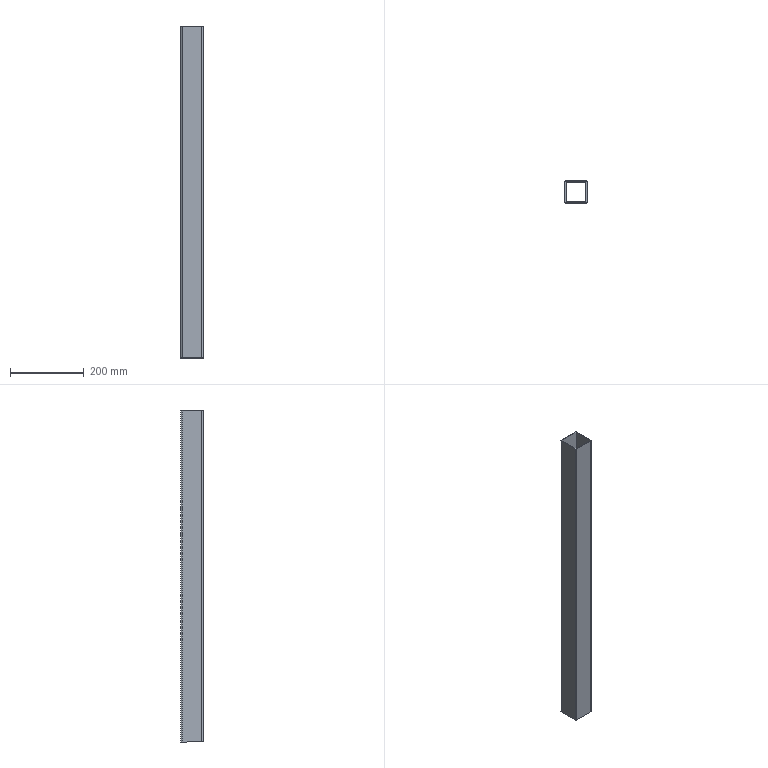Part | STEP file | X77-03102 | 1 solid | 14 faces | box 60 x 60 x 900 mm | volume 608647 mm3 | plane 10 | cylinder 4 | commonest cylinder face diameters 6 x4
STEP:
#1=CARTESIAN_POINT('',(0.,3.,900.));
#2=VERTEX_POINT('',#1);
#3=CARTESIAN_POINT('',(3.,0.,900.));
#4=VERTEX_POINT('',#3);
#5=CARTESIAN_POINT('',(3.,3.,900.));
#6=DIRECTION('',(0.,0.,1.));
#7=DIRECTION('',(1.,0.,0.));
#8=AXIS2_PLACEMENT_3D('',#5,#6,#7);
#9=CIRCLE('',#8,3.);
#10=EDGE_CURVE('',#2,#4,#9,.T.);
#11=ORIENTED_EDGE('',*,*,#10,.T.);
#12=CARTESIAN_POINT('',(57.,0.,900.));
#13=VERTEX_POINT('',#12);
#14=CARTESIAN_POINT('',(3.,0.,900.));
#15=DIRECTION('',(1.,0.,0.));
#16=VECTOR('',#15,1000.);
#17=LINE('',#14,#16);
#18=EDGE_CURVE('',#4,#13,#17,.T.);
#19=ORIENTED_EDGE('',*,*,#18,.T.);
#20=CARTESIAN_POINT('',(60.,3.,900.));
#21=VERTEX_POINT('',#20);
#22=CARTESIAN_POINT('',(57.,3.,900.));
#23=DIRECTION('',(0.,0.,1.));
#24=DIRECTION('',(1.,0.,0.));
#25=AXIS2_PLACEMENT_3D('',#22,#23,#24);
#26=CIRCLE('',#25,3.);
#27=EDGE_CURVE('',#13,#21,#26,.T.);
#28=ORIENTED_EDGE('',*,*,#27,.T.);
#29=CARTESIAN_POINT('',(60.,57.,900.));
#30=VERTEX_POINT('',#29);
#31=CARTESIAN_POINT('',(60.,3.,900.));
#32=DIRECTION('',(0.,1.,0.));
#33=VECTOR('',#32,1000.);
#34=LINE('',#31,#33);
#35=EDGE_CURVE('',#21,#30,#34,.T.);
#36=ORIENTED_EDGE('',*,*,#35,.T.);
#37=CARTESIAN_POINT('',(57.,60.,900.));
#38=VERTEX_POINT('',#37);
#39=CARTESIAN_POINT('',(57.,57.,900.));
#40=DIRECTION('',(0.,0.,1.));
#41=DIRECTION('',(1.,0.,0.));
#42=AXIS2_PLACEMENT_3D('',#39,#40,#41);
#43=CIRCLE('',#42,3.);
#44=EDGE_CURVE('',#30,#38,#43,.T.);
#45=ORIENTED_EDGE('',*,*,#44,.T.);
#46=CARTESIAN_POINT('',(3.,60.,900.));
#47=VERTEX_POINT('',#46);
#48=CARTESIAN_POINT('',(3.,60.,900.));
#49=DIRECTION('',(-1.,0.,0.));
#50=VECTOR('',#49,1000.);
#51=LINE('',#48,#50);
#52=EDGE_CURVE('',#38,#47,#51,.T.);
#53=ORIENTED_EDGE('',*,*,#52,.T.);
#54=CARTESIAN_POINT('',(0.,57.,900.));
#55=VERTEX_POINT('',#54);
#56=CARTESIAN_POINT('',(3.,57.,900.));
#57=DIRECTION('',(0.,0.,1.));
#58=DIRECTION('',(1.,0.,0.));
#59=AXIS2_PLACEMENT_3D('',#56,#57,#58);
#60=CIRCLE('',#59,3.);
#61=EDGE_CURVE('',#47,#55,#60,.T.);
#62=ORIENTED_EDGE('',*,*,#61,.T.);
#63=CARTESIAN_POINT('',(0.,3.,900.));
#64=DIRECTION('',(0.,-1.,0.));
#65=VECTOR('',#64,1000.);
#66=LINE('',#63,#65);
#67=EDGE_CURVE('',#55,#2,#66,.T.);
#68=ORIENTED_EDGE('',*,*,#67,.T.);
#69=EDGE_LOOP('',(#11,#19,#28,#36,#45,#53,#62,#68));
#70=FACE_OUTER_BOUND('',#69,.T.);
#71=CARTESIAN_POINT('',(3.,3.,900.));
#72=VERTEX_POINT('',#71);
#73=CARTESIAN_POINT('',(57.,3.,900.));
#74=VERTEX_POINT('',#73);
#75=CARTESIAN_POINT('',(3.,3.,900.));
#76=DIRECTION('',(1.,0.,0.));
#77=VECTOR('',#76,1000.);
#78=LINE('',#75,#77);
#79=EDGE_CURVE('',#72,#74,#78,.T.);
#80=ORIENTED_EDGE('',*,*,#79,.F.);
#81=CARTESIAN_POINT('',(3.,57.,900.));
#82=VERTEX_POINT('',#81);
#83=CARTESIAN_POINT('',(3.,3.,900.));
#84=DIRECTION('',(0.,-1.,0.));
#85=VECTOR('',#84,1000.);
#86=LINE('',#83,#85);
#87=EDGE_CURVE('',#82,#72,#86,.T.);
#88=ORIENTED_EDGE('',*,*,#87,.F.);
#89=CARTESIAN_POINT('',(57.,57.,900.));
#90=VERTEX_POINT('',#89);
#91=CARTESIAN_POINT('',(3.,57.,900.));
#92=DIRECTION('',(-1.,0.,0.));
#93=VECTOR('',#92,1000.);
#94=LINE('',#91,#93);
#95=EDGE_CURVE('',#90,#82,#94,.T.);
#96=ORIENTED_EDGE('',*,*,#95,.F.);
#97=CARTESIAN_POINT('',(57.,3.,900.));
#98=DIRECTION('',(0.,1.,0.));
#99=VECTOR('',#98,1000.);
#100=LINE('',#97,#99);
#101=EDGE_CURVE('',#74,#90,#100,.T.);
#102=ORIENTED_EDGE('',*,*,#101,.F.);
#103=EDGE_LOOP('',(#80,#88,#96,#102));
#104=FACE_BOUND('',#103,.T.);
#105=CARTESIAN_POINT('',(3.,3.,900.));
#106=DIRECTION('',(0.,0.,1.));
#107=DIRECTION('',(1.,0.,0.));
#108=AXIS2_PLACEMENT_3D('',#105,#106,#107);
#109=PLANE('',#108);
#110=ADVANCED_FACE('',(#70,#104),#109,.T.);
#111=CARTESIAN_POINT('',(0.,3.,0.));
#112=VERTEX_POINT('',#111);
#113=CARTESIAN_POINT('',(3.,0.,0.));
#114=VERTEX_POINT('',#113);
#115=CARTESIAN_POINT('',(3.,3.,0.));
#116=DIRECTION('',(0.,0.,1.));
#117=DIRECTION('',(1.,0.,0.));
#118=AXIS2_PLACEMENT_3D('',#115,#116,#117);
#119=CIRCLE('',#118,3.);
#120=EDGE_CURVE('',#112,#114,#119,.T.);
#121=ORIENTED_EDGE('',*,*,#120,.F.);
#122=CARTESIAN_POINT('',(0.,57.,0.));
#123=VERTEX_POINT('',#122);
#124=CARTESIAN_POINT('',(0.,3.,0.));
#125=DIRECTION('',(0.,-1.,0.));
#126=VECTOR('',#125,1000.);
#127=LINE('',#124,#126);
#128=EDGE_CURVE('',#123,#112,#127,.T.);
#129=ORIENTED_EDGE('',*,*,#128,.F.);
#130=CARTESIAN_POINT('',(3.,60.,0.));
#131=VERTEX_POINT('',#130);
#132=CARTESIAN_POINT('',(3.,57.,0.));
#133=DIRECTION('',(0.,0.,1.));
#134=DIRECTION('',(1.,0.,0.));
#135=AXIS2_PLACEMENT_3D('',#132,#133,#134);
#136=CIRCLE('',#135,3.);
#137=EDGE_CURVE('',#131,#123,#136,.T.);
#138=ORIENTED_EDGE('',*,*,#137,.F.);
#139=CARTESIAN_POINT('',(57.,60.,0.));
#140=VERTEX_POINT('',#139);
#141=CARTESIAN_POINT('',(3.,60.,0.));
#142=DIRECTION('',(-1.,0.,0.));
#143=VECTOR('',#142,1000.);
#144=LINE('',#141,#143);
#145=EDGE_CURVE('',#140,#131,#144,.T.);
#146=ORIENTED_EDGE('',*,*,#145,.F.);
#147=CARTESIAN_POINT('',(60.,57.,0.));
#148=VERTEX_POINT('',#147);
#149=CARTESIAN_POINT('',(57.,57.,0.));
#150=DIRECTION('',(0.,0.,1.));
#151=DIRECTION('',(1.,0.,0.));
#152=AXIS2_PLACEMENT_3D('',#149,#150,#151);
#153=CIRCLE('',#152,3.);
#154=EDGE_CURVE('',#148,#140,#153,.T.);
#155=ORIENTED_EDGE('',*,*,#154,.F.);
#156=CARTESIAN_POINT('',(60.,3.,0.));
#157=VERTEX_POINT('',#156);
#158=CARTESIAN_POINT('',(60.,3.,0.));
#159=DIRECTION('',(0.,1.,0.));
#160=VECTOR('',#159,1000.);
#161=LINE('',#158,#160);
#162=EDGE_CURVE('',#157,#148,#161,.T.);
#163=ORIENTED_EDGE('',*,*,#162,.F.);
#164=CARTESIAN_POINT('',(57.,0.,0.));
#165=VERTEX_POINT('',#164);
#166=CARTESIAN_POINT('',(57.,3.,0.));
#167=DIRECTION('',(0.,0.,1.));
#168=DIRECTION('',(1.,0.,0.));
#169=AXIS2_PLACEMENT_3D('',#166,#167,#168);
#170=CIRCLE('',#169,3.);
#171=EDGE_CURVE('',#165,#157,#170,.T.);
#172=ORIENTED_EDGE('',*,*,#171,.F.);
#173=CARTESIAN_POINT('',(3.,0.,0.));
#174=DIRECTION('',(1.,0.,0.));
#175=VECTOR('',#174,1000.);
#176=LINE('',#173,#175);
#177=EDGE_CURVE('',#114,#165,#176,.T.);
#178=ORIENTED_EDGE('',*,*,#177,.F.);
#179=EDGE_LOOP('',(#121,#129,#138,#146,#155,#163,#172,#178));
#180=FACE_OUTER_BOUND('',#179,.T.);
#181=CARTESIAN_POINT('',(3.,57.,0.));
#182=VERTEX_POINT('',#181);
#183=CARTESIAN_POINT('',(3.,3.,0.));
#184=VERTEX_POINT('',#183);
#185=CARTESIAN_POINT('',(3.,3.,0.));
#186=DIRECTION('',(0.,-1.,0.));
#187=VECTOR('',#186,1000.);
#188=LINE('',#185,#187);
#189=EDGE_CURVE('',#182,#184,#188,.T.);
#190=ORIENTED_EDGE('',*,*,#189,.T.);
#191=CARTESIAN_POINT('',(57.,3.,0.));
#192=VERTEX_POINT('',#191);
#193=CARTESIAN_POINT('',(3.,3.,0.));
#194=DIRECTION('',(1.,0.,0.));
#195=VECTOR('',#194,1000.);
#196=LINE('',#193,#195);
#197=EDGE_CURVE('',#184,#192,#196,.T.);
#198=ORIENTED_EDGE('',*,*,#197,.T.);
#199=CARTESIAN_POINT('',(57.,57.,0.));
#200=VERTEX_POINT('',#199);
#201=CARTESIAN_POINT('',(57.,3.,0.));
#202=DIRECTION('',(0.,1.,0.));
#203=VECTOR('',#202,1000.);
#204=LINE('',#201,#203);
#205=EDGE_CURVE('',#192,#200,#204,.T.);
#206=ORIENTED_EDGE('',*,*,#205,.T.);
#207=CARTESIAN_POINT('',(3.,57.,0.));
#208=DIRECTION('',(-1.,0.,0.));
#209=VECTOR('',#208,1000.);
#210=LINE('',#207,#209);
#211=EDGE_CURVE('',#200,#182,#210,.T.);
#212=ORIENTED_EDGE('',*,*,#211,.T.);
#213=EDGE_LOOP('',(#190,#198,#206,#212));
#214=FACE_BOUND('',#213,.T.);
#215=CARTESIAN_POINT('',(3.,3.,0.));
#216=DIRECTION('',(0.,0.,1.));
#217=DIRECTION('',(1.,0.,0.));
#218=AXIS2_PLACEMENT_3D('',#215,#216,#217);
#219=PLANE('',#218);
#220=ADVANCED_FACE('',(#180,#214),#219,.F.);
#221=ORIENTED_EDGE('',*,*,#120,.T.);
#222=CARTESIAN_POINT('',(3.,0.,900.));
#223=DIRECTION('',(0.,0.,-1.));
#224=VECTOR('',#223,1000.);
#225=LINE('',#222,#224);
#226=EDGE_CURVE('',#4,#114,#225,.T.);
#227=ORIENTED_EDGE('',*,*,#226,.F.);
#228=ORIENTED_EDGE('',*,*,#10,.F.);
#229=CARTESIAN_POINT('',(0.,3.,900.));
#230=DIRECTION('',(0.,0.,-1.));
#231=VECTOR('',#230,1000.);
#232=LINE('',#229,#231);
#233=EDGE_CURVE('',#2,#112,#232,.T.);
#234=ORIENTED_EDGE('',*,*,#233,.T.);
#235=EDGE_LOOP('',(#221,#227,#228,#234));
#236=FACE_OUTER_BOUND('',#235,.T.);
#237=CARTESIAN_POINT('',(3.,3.,900.));
#238=DIRECTION('',(0.,0.,-1.));
#239=DIRECTION('',(-1.,0.,0.));
#240=AXIS2_PLACEMENT_3D('',#237,#238,#239);
#241=CYLINDRICAL_SURFACE('',#240,3.);
#242=ADVANCED_FACE('',(#236),#241,.T.);
#243=ORIENTED_EDGE('',*,*,#177,.T.);
#244=CARTESIAN_POINT('',(57.,0.,900.));
#245=DIRECTION('',(0.,0.,-1.));
#246=VECTOR('',#245,1000.);
#247=LINE('',#244,#246);
#248=EDGE_CURVE('',#13,#165,#247,.T.);
#249=ORIENTED_EDGE('',*,*,#248,.F.);
#250=ORIENTED_EDGE('',*,*,#18,.F.);
#251=ORIENTED_EDGE('',*,*,#226,.T.);
#252=EDGE_LOOP('',(#243,#249,#250,#251));
#253=FACE_OUTER_BOUND('',#252,.T.);
#254=CARTESIAN_POINT('',(3.,0.,900.));
#255=DIRECTION('',(0.,1.,0.));
#256=DIRECTION('',(0.,0.,1.));
#257=AXIS2_PLACEMENT_3D('',#254,#255,#256);
#258=PLANE('',#257);
#259=ADVANCED_FACE('',(#253),#258,.F.);
#260=ORIENTED_EDGE('',*,*,#171,.T.);
#261=CARTESIAN_POINT('',(60.,3.,900.));
#262=DIRECTION('',(0.,0.,-1.));
#263=VECTOR('',#262,1000.);
#264=LINE('',#261,#263);
#265=EDGE_CURVE('',#21,#157,#264,.T.);
#266=ORIENTED_EDGE('',*,*,#265,.F.);
#267=ORIENTED_EDGE('',*,*,#27,.F.);
#268=ORIENTED_EDGE('',*,*,#248,.T.);
#269=EDGE_LOOP('',(#260,#266,#267,#268));
#270=FACE_OUTER_BOUND('',#269,.T.);
#271=CARTESIAN_POINT('',(57.,3.,900.));
#272=DIRECTION('',(0.,0.,-1.));
#273=DIRECTION('',(-1.,0.,0.));
#274=AXIS2_PLACEMENT_3D('',#271,#272,#273);
#275=CYLINDRICAL_SURFACE('',#274,3.);
#276=ADVANCED_FACE('',(#270),#275,.T.);
#277=ORIENTED_EDGE('',*,*,#162,.T.);
#278=CARTESIAN_POINT('',(60.,57.,900.));
#279=DIRECTION('',(0.,0.,-1.));
#280=VECTOR('',#279,1000.);
#281=LINE('',#278,#280);
#282=EDGE_CURVE('',#30,#148,#281,.T.);
#283=ORIENTED_EDGE('',*,*,#282,.F.);
#284=ORIENTED_EDGE('',*,*,#35,.F.);
#285=ORIENTED_EDGE('',*,*,#265,.T.);
#286=EDGE_LOOP('',(#277,#283,#284,#285));
#287=FACE_OUTER_BOUND('',#286,.T.);
#288=CARTESIAN_POINT('',(60.,3.,900.));
#289=DIRECTION('',(-1.,0.,0.));
#290=DIRECTION('',(0.,0.,1.));
#291=AXIS2_PLACEMENT_3D('',#288,#289,#290);
#292=PLANE('',#291);
#293=ADVANCED_FACE('',(#287),#292,.F.);
#294=ORIENTED_EDGE('',*,*,#154,.T.);
#295=CARTESIAN_POINT('',(57.,60.,900.));
#296=DIRECTION('',(0.,0.,-1.));
#297=VECTOR('',#296,1000.);
#298=LINE('',#295,#297);
#299=EDGE_CURVE('',#38,#140,#298,.T.);
#300=ORIENTED_EDGE('',*,*,#299,.F.);
#301=ORIENTED_EDGE('',*,*,#44,.F.);
#302=ORIENTED_EDGE('',*,*,#282,.T.);
#303=EDGE_LOOP('',(#294,#300,#301,#302));
#304=FACE_OUTER_BOUND('',#303,.T.);
#305=CARTESIAN_POINT('',(57.,57.,900.));
#306=DIRECTION('',(0.,0.,-1.));
#307=DIRECTION('',(-1.,0.,0.));
#308=AXIS2_PLACEMENT_3D('',#305,#306,#307);
#309=CYLINDRICAL_SURFACE('',#308,3.);
#310=ADVANCED_FACE('',(#304),#309,.T.);
#311=ORIENTED_EDGE('',*,*,#145,.T.);
#312=CARTESIAN_POINT('',(3.,60.,900.));
#313=DIRECTION('',(0.,0.,-1.));
#314=VECTOR('',#313,1000.);
#315=LINE('',#312,#314);
#316=EDGE_CURVE('',#47,#131,#315,.T.);
#317=ORIENTED_EDGE('',*,*,#316,.F.);
#318=ORIENTED_EDGE('',*,*,#52,.F.);
#319=ORIENTED_EDGE('',*,*,#299,.T.);
#320=EDGE_LOOP('',(#311,#317,#318,#319));
#321=FACE_OUTER_BOUND('',#320,.T.);
#322=CARTESIAN_POINT('',(3.,60.,900.));
#323=DIRECTION('',(0.,-1.,0.));
#324=DIRECTION('',(0.,0.,-1.));
#325=AXIS2_PLACEMENT_3D('',#322,#323,#324);
#326=PLANE('',#325);
#327=ADVANCED_FACE('',(#321),#326,.F.);
#328=ORIENTED_EDGE('',*,*,#137,.T.);
#329=CARTESIAN_POINT('',(0.,57.,900.));
#330=DIRECTION('',(0.,0.,-1.));
#331=VECTOR('',#330,1000.);
#332=LINE('',#329,#331);
#333=EDGE_CURVE('',#55,#123,#332,.T.);
#334=ORIENTED_EDGE('',*,*,#333,.F.);
#335=ORIENTED_EDGE('',*,*,#61,.F.);
#336=ORIENTED_EDGE('',*,*,#316,.T.);
#337=EDGE_LOOP('',(#328,#334,#335,#336));
#338=FACE_OUTER_BOUND('',#337,.T.);
#339=CARTESIAN_POINT('',(3.,57.,900.));
#340=DIRECTION('',(0.,0.,-1.));
#341=DIRECTION('',(-1.,0.,0.));
#342=AXIS2_PLACEMENT_3D('',#339,#340,#341);
#343=CYLINDRICAL_SURFACE('',#342,3.);
#344=ADVANCED_FACE('',(#338),#343,.T.);
#345=ORIENTED_EDGE('',*,*,#128,.T.);
#346=ORIENTED_EDGE('',*,*,#233,.F.);
#347=ORIENTED_EDGE('',*,*,#67,.F.);
#348=ORIENTED_EDGE('',*,*,#333,.T.);
#349=EDGE_LOOP('',(#345,#346,#347,#348));
#350=FACE_OUTER_BOUND('',#349,.T.);
#351=CARTESIAN_POINT('',(0.,3.,900.));
#352=DIRECTION('',(1.,0.,0.));
#353=DIRECTION('',(0.,0.,-1.));
#354=AXIS2_PLACEMENT_3D('',#351,#352,#353);
#355=PLANE('',#354);
#356=ADVANCED_FACE('',(#350),#355,.F.);
#357=ORIENTED_EDGE('',*,*,#189,.F.);
#358=CARTESIAN_POINT('',(3.,57.,900.));
#359=DIRECTION('',(0.,0.,-1.));
#360=VECTOR('',#359,1000.);
#361=LINE('',#358,#360);
#362=EDGE_CURVE('',#82,#182,#361,.T.);
#363=ORIENTED_EDGE('',*,*,#362,.F.);
#364=ORIENTED_EDGE('',*,*,#87,.T.);
#365=CARTESIAN_POINT('',(3.,3.,900.));
#366=DIRECTION('',(0.,0.,-1.));
#367=VECTOR('',#366,1000.);
#368=LINE('',#365,#367);
#369=EDGE_CURVE('',#72,#184,#368,.T.);
#370=ORIENTED_EDGE('',*,*,#369,.T.);
#371=EDGE_LOOP('',(#357,#363,#364,#370));
#372=FACE_OUTER_BOUND('',#371,.T.);
#373=CARTESIAN_POINT('',(3.,3.,900.));
#374=DIRECTION('',(1.,0.,0.));
#375=DIRECTION('',(0.,0.,-1.));
#376=AXIS2_PLACEMENT_3D('',#373,#374,#375);
#377=PLANE('',#376);
#378=ADVANCED_FACE('',(#372),#377,.T.);
#379=ORIENTED_EDGE('',*,*,#197,.F.);
#380=ORIENTED_EDGE('',*,*,#369,.F.);
#381=ORIENTED_EDGE('',*,*,#79,.T.);
#382=CARTESIAN_POINT('',(57.,3.,900.));
#383=DIRECTION('',(0.,0.,-1.));
#384=VECTOR('',#383,1000.);
#385=LINE('',#382,#384);
#386=EDGE_CURVE('',#74,#192,#385,.T.);
#387=ORIENTED_EDGE('',*,*,#386,.T.);
#388=EDGE_LOOP('',(#379,#380,#381,#387));
#389=FACE_OUTER_BOUND('',#388,.T.);
#390=CARTESIAN_POINT('',(3.,3.,900.));
#391=DIRECTION('',(0.,1.,0.));
#392=DIRECTION('',(0.,0.,1.));
#393=AXIS2_PLACEMENT_3D('',#390,#391,#392);
#394=PLANE('',#393);
#395=ADVANCED_FACE('',(#389),#394,.T.);
#396=ORIENTED_EDGE('',*,*,#205,.F.);
#397=ORIENTED_EDGE('',*,*,#386,.F.);
#398=ORIENTED_EDGE('',*,*,#101,.T.);
#399=CARTESIAN_POINT('',(57.,57.,900.));
#400=DIRECTION('',(0.,0.,-1.));
#401=VECTOR('',#400,1000.);
#402=LINE('',#399,#401);
#403=EDGE_CURVE('',#90,#200,#402,.T.);
#404=ORIENTED_EDGE('',*,*,#403,.T.);
#405=EDGE_LOOP('',(#396,#397,#398,#404));
#406=FACE_OUTER_BOUND('',#405,.T.);
#407=CARTESIAN_POINT('',(57.,3.,900.));
#408=DIRECTION('',(-1.,0.,0.));
#409=DIRECTION('',(0.,0.,1.));
#410=AXIS2_PLACEMENT_3D('',#407,#408,#409);
#411=PLANE('',#410);
#412=ADVANCED_FACE('',(#406),#411,.T.);
#413=ORIENTED_EDGE('',*,*,#211,.F.);
#414=ORIENTED_EDGE('',*,*,#403,.F.);
#415=ORIENTED_EDGE('',*,*,#95,.T.);
#416=ORIENTED_EDGE('',*,*,#362,.T.);
#417=EDGE_LOOP('',(#413,#414,#415,#416));
#418=FACE_OUTER_BOUND('',#417,.T.);
#419=CARTESIAN_POINT('',(3.,57.,900.));
#420=DIRECTION('',(0.,-1.,0.));
#421=DIRECTION('',(0.,0.,-1.));
#422=AXIS2_PLACEMENT_3D('',#419,#420,#421);
#423=PLANE('',#422);
#424=ADVANCED_FACE('',(#418),#423,.T.);
#425=CLOSED_SHELL('',(#110,#220,#242,#259,#276,#293,#310,#327,#344,#356,#378,#395,#412,#424));
#426=MANIFOLD_SOLID_BREP('',#425);
#427=CARTESIAN_POINT('',(0.,0.,0.));
#428=DIRECTION('',(0.,0.,1.));
#429=DIRECTION('',(1.,0.,0.));
#430=AXIS2_PLACEMENT_3D('',#427,#428,#429);
#431=(LENGTH_UNIT()NAMED_UNIT(*)SI_UNIT(.MILLI.,.METRE.));
#432=UNCERTAINTY_MEASURE_WITH_UNIT(LENGTH_MEASURE(0.00001),#431,'','');
#433=(NAMED_UNIT(*)PLANE_ANGLE_UNIT()SI_UNIT($,.RADIAN.));
#434=(NAMED_UNIT(*)SI_UNIT($,.STERADIAN.)SOLID_ANGLE_UNIT());
#435=(GEOMETRIC_REPRESENTATION_CONTEXT(3)GLOBAL_UNCERTAINTY_ASSIGNED_CONTEXT((#432))GLOBAL_UNIT_ASSIGNED_CONTEXT((#431,#433,#434))REPRESENTATION_CONTEXT('',''));
#436=ADVANCED_BREP_SHAPE_REPRESENTATION('',(#426,#430),#435);